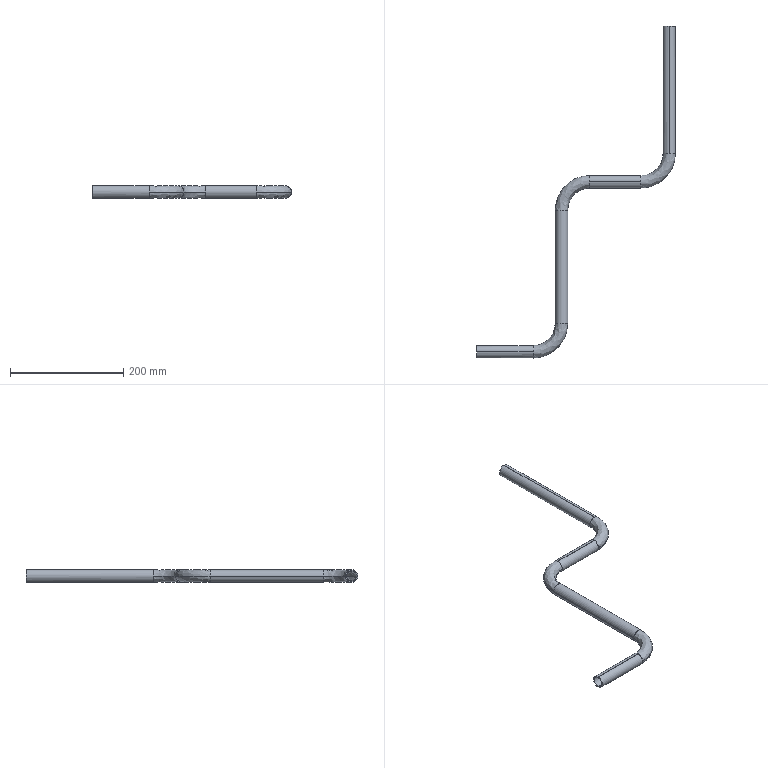Part | STEP file | copper tube 21_default_machined_ | 1 solid | 30 faces | box 351.2 x 586 x 22 mm | volume 82193 mm3 | cylinder 16 | spline 12 | plane 2 | commonest cylinder face diameters 19 x8 22 x8